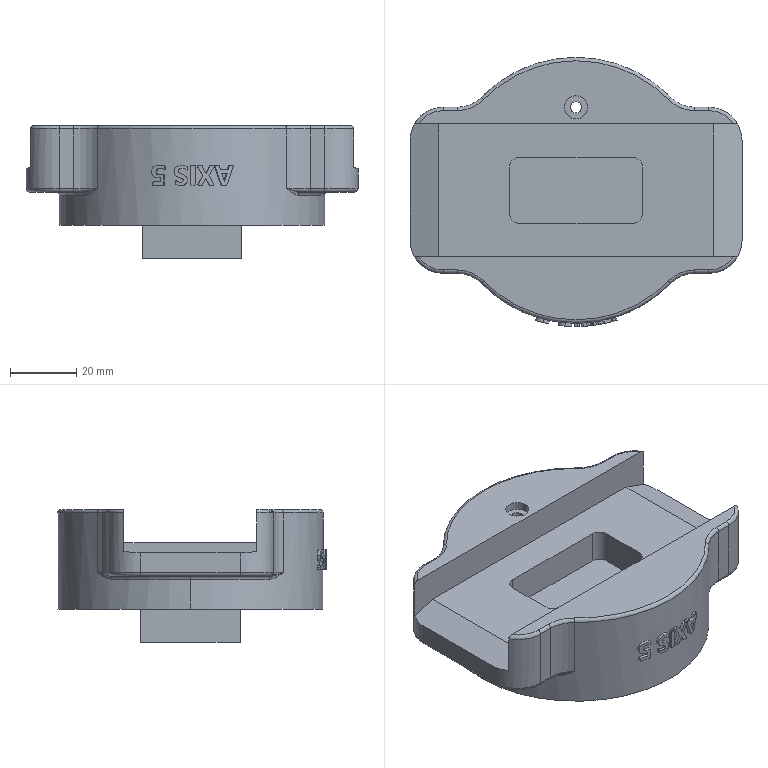Part | SolidWorks | features ICE 4, Fillet 3, 3DProfileFeature 1, Chamfer 1, Emboss 1, Extrusion 1, HoleWzd 1 | 1 solid | 152 faces | box 100 x 81 x 40 mm | volume 134637 mm3 | spline 61 | plane 36 | cylinder 34 | torus 21 | commonest cylinder face diameters 2 x10 20 x8 82 x5 6 x4 80 x3 3.4 x2